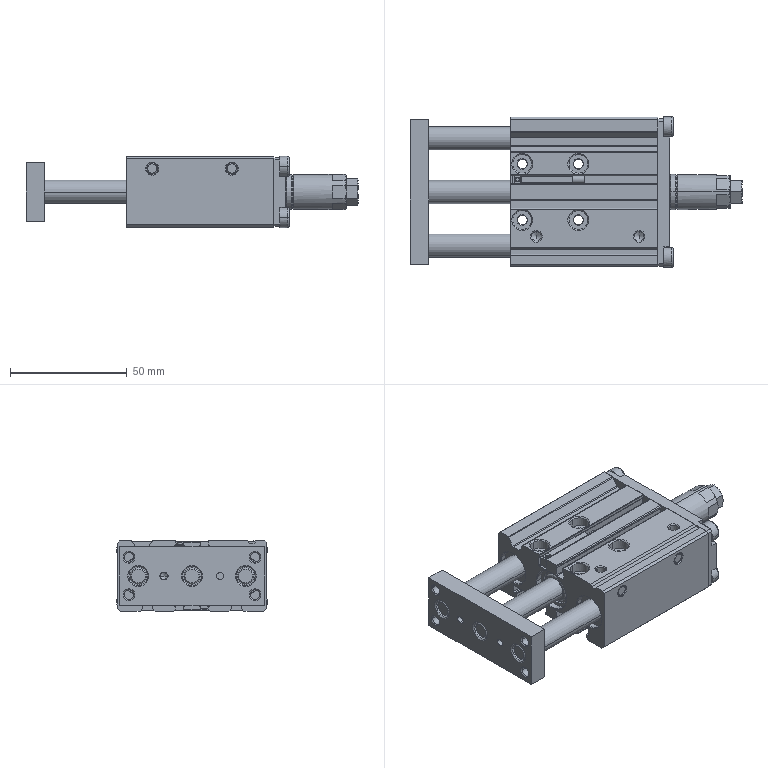Part | SolidWorks | features BaseBody 5, MoveFace 1 | 5 solids | 618 faces | box 142 x 64.5 x 30.5 mm | volume 123936 mm3 | plane 240 | cylinder 225 | cone 143 | spline 10 | commonest cylinder face diameters 4.134 x28 3 x25 0.4 x20 0.8 x20 8 x14 10 x14